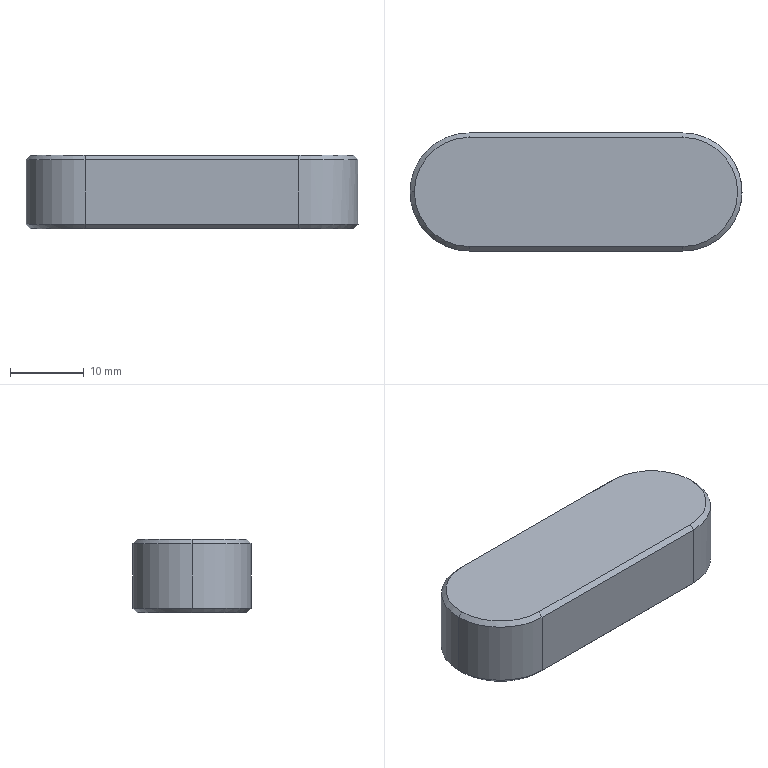Part | SolidWorks | features Boss 2, Chamfer 1, Extrusion 1 | 1 solid | 17 faces | box 45 x 16 x 10 mm | volume 6612 mm3 | plane 8 | cone 6 | cylinder 3 | commonest cylinder face diameters 16 x3
STEP:
#1=CARTESIAN_POINT('',(-36.4,0.,5.));
#2=VERTEX_POINT('',#1);
#3=CARTESIAN_POINT('',(-29.,-7.4,5.));
#4=VERTEX_POINT('',#3);
#5=CARTESIAN_POINT('',(-29.,0.,5.));
#6=DIRECTION('',(0.,0.,1.));
#7=DIRECTION('',(-1.,0.,0.));
#8=AXIS2_PLACEMENT_3D('',#5,#6,#7);
#9=CIRCLE('',#8,7.4);
#10=EDGE_CURVE('',#2,#4,#9,.T.);
#11=ORIENTED_EDGE('',*,*,#10,.F.);
#12=CARTESIAN_POINT('',(-37.,0.,4.4));
#13=VERTEX_POINT('',#12);
#14=CARTESIAN_POINT('',(-36.4,0.,5.));
#15=DIRECTION('',(-0.7071,0.,-0.7071));
#16=VECTOR('',#15,1000.);
#17=LINE('',#14,#16);
#18=EDGE_CURVE('',#2,#13,#17,.T.);
#19=ORIENTED_EDGE('',*,*,#18,.T.);
#20=CARTESIAN_POINT('',(-29.,-8.,4.4));
#21=VERTEX_POINT('',#20);
#22=CARTESIAN_POINT('',(-29.,0.,4.4));
#23=DIRECTION('',(0.,0.,-1.));
#24=DIRECTION('',(-1.,0.,0.));
#25=AXIS2_PLACEMENT_3D('',#22,#23,#24);
#26=CIRCLE('',#25,8.);
#27=EDGE_CURVE('',#21,#13,#26,.T.);
#28=ORIENTED_EDGE('',*,*,#27,.F.);
#29=CARTESIAN_POINT('',(-29.,-7.4,5.));
#30=DIRECTION('',(0.,-0.7071,-0.7071));
#31=VECTOR('',#30,1000.);
#32=LINE('',#29,#31);
#33=EDGE_CURVE('',#4,#21,#32,.T.);
#34=ORIENTED_EDGE('',*,*,#33,.F.);
#35=EDGE_LOOP('',(#11,#19,#28,#34));
#36=FACE_OUTER_BOUND('',#35,.T.);
#37=CARTESIAN_POINT('',(-29.,0.,5.));
#38=DIRECTION('',(0.,0.,-1.));
#39=DIRECTION('',(-1.,0.,0.));
#40=AXIS2_PLACEMENT_3D('',#37,#38,#39);
#41=CONICAL_SURFACE('',#40,7.4,0.7854);
#42=ADVANCED_FACE('',(#36),#41,.T.);
#43=CARTESIAN_POINT('',(7.4,0.,-5.));
#44=VERTEX_POINT('',#43);
#45=CARTESIAN_POINT('',(0.,-7.4,-5.));
#46=VERTEX_POINT('',#45);
#47=CARTESIAN_POINT('',(0.,0.,-5.));
#48=DIRECTION('',(0.,0.,-1.));
#49=DIRECTION('',(-1.,0.,0.));
#50=AXIS2_PLACEMENT_3D('',#47,#48,#49);
#51=CIRCLE('',#50,7.4);
#52=EDGE_CURVE('',#44,#46,#51,.T.);
#53=ORIENTED_EDGE('',*,*,#52,.F.);
#54=CARTESIAN_POINT('',(8.,0.,-4.4));
#55=VERTEX_POINT('',#54);
#56=CARTESIAN_POINT('',(8.,0.,-4.4));
#57=DIRECTION('',(0.7071,0.,0.7071));
#58=VECTOR('',#57,1000.);
#59=LINE('',#56,#58);
#60=EDGE_CURVE('',#44,#55,#59,.T.);
#61=ORIENTED_EDGE('',*,*,#60,.T.);
#62=CARTESIAN_POINT('',(0.,-8.,-4.4));
#63=VERTEX_POINT('',#62);
#64=CARTESIAN_POINT('',(0.,0.,-4.4));
#65=DIRECTION('',(0.,0.,1.));
#66=DIRECTION('',(-1.,0.,0.));
#67=AXIS2_PLACEMENT_3D('',#64,#65,#66);
#68=CIRCLE('',#67,8.);
#69=EDGE_CURVE('',#63,#55,#68,.T.);
#70=ORIENTED_EDGE('',*,*,#69,.F.);
#71=CARTESIAN_POINT('',(0.,-7.4,-5.));
#72=DIRECTION('',(0.,-0.7071,0.7071));
#73=VECTOR('',#72,1000.);
#74=LINE('',#71,#73);
#75=EDGE_CURVE('',#46,#63,#74,.T.);
#76=ORIENTED_EDGE('',*,*,#75,.F.);
#77=EDGE_LOOP('',(#53,#61,#70,#76));
#78=FACE_OUTER_BOUND('',#77,.T.);
#79=CARTESIAN_POINT('',(0.,0.,-4.4));
#80=DIRECTION('',(0.,0.,1.));
#81=DIRECTION('',(1.,0.,0.));
#82=AXIS2_PLACEMENT_3D('',#79,#80,#81);
#83=CONICAL_SURFACE('',#82,8.,0.7854);
#84=ADVANCED_FACE('',(#78),#83,.T.);
#85=ORIENTED_EDGE('',*,*,#27,.T.);
#86=CARTESIAN_POINT('',(-37.,0.,-4.4));
#87=VERTEX_POINT('',#86);
#88=CARTESIAN_POINT('',(-37.,0.,5.));
#89=DIRECTION('',(0.,0.,-1.));
#90=VECTOR('',#89,1000.);
#91=LINE('',#88,#90);
#92=EDGE_CURVE('',#13,#87,#91,.T.);
#93=ORIENTED_EDGE('',*,*,#92,.T.);
#94=CARTESIAN_POINT('',(-29.,-8.,-4.4));
#95=VERTEX_POINT('',#94);
#96=CARTESIAN_POINT('',(-29.,0.,-4.4));
#97=DIRECTION('',(0.,0.,1.));
#98=DIRECTION('',(-1.,0.,0.));
#99=AXIS2_PLACEMENT_3D('',#96,#97,#98);
#100=CIRCLE('',#99,8.);
#101=EDGE_CURVE('',#87,#95,#100,.T.);
#102=ORIENTED_EDGE('',*,*,#101,.T.);
#103=CARTESIAN_POINT('',(-29.,-8.,5.));
#104=DIRECTION('',(0.,0.,-1.));
#105=VECTOR('',#104,1000.);
#106=LINE('',#103,#105);
#107=EDGE_CURVE('',#21,#95,#106,.T.);
#108=ORIENTED_EDGE('',*,*,#107,.F.);
#109=EDGE_LOOP('',(#85,#93,#102,#108));
#110=FACE_OUTER_BOUND('',#109,.T.);
#111=CARTESIAN_POINT('',(-29.,0.,5.));
#112=DIRECTION('',(0.,0.,-1.));
#113=DIRECTION('',(-1.,0.,0.));
#114=AXIS2_PLACEMENT_3D('',#111,#112,#113);
#115=CYLINDRICAL_SURFACE('',#114,8.);
#116=ADVANCED_FACE('',(#110),#115,.T.);
#117=ORIENTED_EDGE('',*,*,#92,.F.);
#118=CARTESIAN_POINT('',(-29.,8.,4.4));
#119=VERTEX_POINT('',#118);
#120=CARTESIAN_POINT('',(-29.,0.,4.4));
#121=DIRECTION('',(0.,0.,-1.));
#122=DIRECTION('',(-1.,0.,0.));
#123=AXIS2_PLACEMENT_3D('',#120,#121,#122);
#124=CIRCLE('',#123,8.);
#125=EDGE_CURVE('',#13,#119,#124,.T.);
#126=ORIENTED_EDGE('',*,*,#125,.T.);
#127=CARTESIAN_POINT('',(-29.,8.,-4.4));
#128=VERTEX_POINT('',#127);
#129=CARTESIAN_POINT('',(-29.,8.,5.));
#130=DIRECTION('',(0.,0.,-1.));
#131=VECTOR('',#130,1000.);
#132=LINE('',#129,#131);
#133=EDGE_CURVE('',#119,#128,#132,.T.);
#134=ORIENTED_EDGE('',*,*,#133,.T.);
#135=CARTESIAN_POINT('',(-29.,0.,-4.4));
#136=DIRECTION('',(0.,0.,1.));
#137=DIRECTION('',(-1.,0.,0.));
#138=AXIS2_PLACEMENT_3D('',#135,#136,#137);
#139=CIRCLE('',#138,8.);
#140=EDGE_CURVE('',#128,#87,#139,.T.);
#141=ORIENTED_EDGE('',*,*,#140,.T.);
#142=EDGE_LOOP('',(#117,#126,#134,#141));
#143=FACE_OUTER_BOUND('',#142,.T.);
#144=CARTESIAN_POINT('',(-29.,0.,5.));
#145=DIRECTION('',(0.,0.,-1.));
#146=DIRECTION('',(-1.,0.,0.));
#147=AXIS2_PLACEMENT_3D('',#144,#145,#146);
#148=CYLINDRICAL_SURFACE('',#147,8.);
#149=ADVANCED_FACE('',(#143),#148,.T.);
#150=ORIENTED_EDGE('',*,*,#107,.T.);
#151=CARTESIAN_POINT('',(0.,-8.,-4.4));
#152=DIRECTION('',(1.,0.,0.));
#153=VECTOR('',#152,1000.);
#154=LINE('',#151,#153);
#155=EDGE_CURVE('',#95,#63,#154,.T.);
#156=ORIENTED_EDGE('',*,*,#155,.T.);
#157=CARTESIAN_POINT('',(0.,-8.,4.4));
#158=VERTEX_POINT('',#157);
#159=CARTESIAN_POINT('',(0.,-8.,5.));
#160=DIRECTION('',(0.,0.,-1.));
#161=VECTOR('',#160,1000.);
#162=LINE('',#159,#161);
#163=EDGE_CURVE('',#158,#63,#162,.T.);
#164=ORIENTED_EDGE('',*,*,#163,.F.);
#165=CARTESIAN_POINT('',(0.,-8.,4.4));
#166=DIRECTION('',(-1.,0.,0.));
#167=VECTOR('',#166,1000.);
#168=LINE('',#165,#167);
#169=EDGE_CURVE('',#158,#21,#168,.T.);
#170=ORIENTED_EDGE('',*,*,#169,.T.);
#171=EDGE_LOOP('',(#150,#156,#164,#170));
#172=FACE_OUTER_BOUND('',#171,.T.);
#173=CARTESIAN_POINT('',(0.,-8.,5.));
#174=DIRECTION('',(0.,1.,0.));
#175=DIRECTION('',(-1.,0.,0.));
#176=AXIS2_PLACEMENT_3D('',#173,#174,#175);
#177=PLANE('',#176);
#178=ADVANCED_FACE('',(#172),#177,.F.);
#179=CARTESIAN_POINT('',(0.,8.,4.4));
#180=VERTEX_POINT('',#179);
#181=CARTESIAN_POINT('',(0.,8.,-4.4));
#182=VERTEX_POINT('',#181);
#183=CARTESIAN_POINT('',(0.,8.,5.));
#184=DIRECTION('',(0.,0.,-1.));
#185=VECTOR('',#184,1000.);
#186=LINE('',#183,#185);
#187=EDGE_CURVE('',#180,#182,#186,.T.);
#188=ORIENTED_EDGE('',*,*,#187,.F.);
#189=CARTESIAN_POINT('',(0.,0.,4.4));
#190=DIRECTION('',(0.,0.,-1.));
#191=DIRECTION('',(-1.,0.,0.));
#192=AXIS2_PLACEMENT_3D('',#189,#190,#191);
#193=CIRCLE('',#192,8.);
#194=EDGE_CURVE('',#180,#158,#193,.T.);
#195=ORIENTED_EDGE('',*,*,#194,.T.);
#196=ORIENTED_EDGE('',*,*,#163,.T.);
#197=ORIENTED_EDGE('',*,*,#69,.T.);
#198=CARTESIAN_POINT('',(0.,0.,-4.4));
#199=DIRECTION('',(0.,0.,1.));
#200=DIRECTION('',(-1.,0.,0.));
#201=AXIS2_PLACEMENT_3D('',#198,#199,#200);
#202=CIRCLE('',#201,8.);
#203=EDGE_CURVE('',#55,#182,#202,.T.);
#204=ORIENTED_EDGE('',*,*,#203,.T.);
#205=EDGE_LOOP('',(#188,#195,#196,#197,#204));
#206=FACE_OUTER_BOUND('',#205,.T.);
#207=CARTESIAN_POINT('',(0.,0.,5.));
#208=DIRECTION('',(0.,0.,-1.));
#209=DIRECTION('',(-1.,0.,0.));
#210=AXIS2_PLACEMENT_3D('',#207,#208,#209);
#211=CYLINDRICAL_SURFACE('',#210,8.);
#212=ADVANCED_FACE('',(#206),#211,.T.);
#213=ORIENTED_EDGE('',*,*,#133,.F.);
#214=CARTESIAN_POINT('',(-29.,8.,4.4));
#215=DIRECTION('',(1.,0.,0.));
#216=VECTOR('',#215,1000.);
#217=LINE('',#214,#216);
#218=EDGE_CURVE('',#119,#180,#217,.T.);
#219=ORIENTED_EDGE('',*,*,#218,.T.);
#220=ORIENTED_EDGE('',*,*,#187,.T.);
#221=CARTESIAN_POINT('',(-29.,8.,-4.4));
#222=DIRECTION('',(-1.,0.,0.));
#223=VECTOR('',#222,1000.);
#224=LINE('',#221,#223);
#225=EDGE_CURVE('',#182,#128,#224,.T.);
#226=ORIENTED_EDGE('',*,*,#225,.T.);
#227=EDGE_LOOP('',(#213,#219,#220,#226));
#228=FACE_OUTER_BOUND('',#227,.T.);
#229=CARTESIAN_POINT('',(-29.,8.,5.));
#230=DIRECTION('',(0.,-1.,0.));
#231=DIRECTION('',(0.,0.,-1.));
#232=AXIS2_PLACEMENT_3D('',#229,#230,#231);
#233=PLANE('',#232);
#234=ADVANCED_FACE('',(#228),#233,.F.);
#235=CARTESIAN_POINT('',(-29.,7.4,5.));
#236=VERTEX_POINT('',#235);
#237=CARTESIAN_POINT('',(-29.,0.,5.));
#238=DIRECTION('',(0.,0.,1.));
#239=DIRECTION('',(-1.,0.,0.));
#240=AXIS2_PLACEMENT_3D('',#237,#238,#239);
#241=CIRCLE('',#240,7.4);
#242=EDGE_CURVE('',#236,#2,#241,.T.);
#243=ORIENTED_EDGE('',*,*,#242,.T.);
#244=ORIENTED_EDGE('',*,*,#10,.T.);
#245=CARTESIAN_POINT('',(0.,-7.4,5.));
#246=VERTEX_POINT('',#245);
#247=CARTESIAN_POINT('',(-29.,-7.4,5.));
#248=DIRECTION('',(1.,0.,0.));
#249=VECTOR('',#248,1000.);
#250=LINE('',#247,#249);
#251=EDGE_CURVE('',#4,#246,#250,.T.);
#252=ORIENTED_EDGE('',*,*,#251,.T.);
#253=CARTESIAN_POINT('',(0.,7.4,5.));
#254=VERTEX_POINT('',#253);
#255=CARTESIAN_POINT('',(0.,0.,5.));
#256=DIRECTION('',(0.,0.,1.));
#257=DIRECTION('',(-1.,0.,0.));
#258=AXIS2_PLACEMENT_3D('',#255,#256,#257);
#259=CIRCLE('',#258,7.4);
#260=EDGE_CURVE('',#246,#254,#259,.T.);
#261=ORIENTED_EDGE('',*,*,#260,.T.);
#262=CARTESIAN_POINT('',(-29.,7.4,5.));
#263=DIRECTION('',(-1.,0.,0.));
#264=VECTOR('',#263,1000.);
#265=LINE('',#262,#264);
#266=EDGE_CURVE('',#254,#236,#265,.T.);
#267=ORIENTED_EDGE('',*,*,#266,.T.);
#268=EDGE_LOOP('',(#243,#244,#252,#261,#267));
#269=FACE_OUTER_BOUND('',#268,.T.);
#270=CARTESIAN_POINT('',(-29.,0.,5.));
#271=DIRECTION('',(0.,0.,-1.));
#272=DIRECTION('',(-1.,0.,0.));
#273=AXIS2_PLACEMENT_3D('',#270,#271,#272);
#274=PLANE('',#273);
#275=ADVANCED_FACE('',(#269),#274,.F.);
#276=CARTESIAN_POINT('',(0.,7.4,-5.));
#277=VERTEX_POINT('',#276);
#278=CARTESIAN_POINT('',(0.,0.,-5.));
#279=DIRECTION('',(0.,0.,-1.));
#280=DIRECTION('',(-1.,0.,0.));
#281=AXIS2_PLACEMENT_3D('',#278,#279,#280);
#282=CIRCLE('',#281,7.4);
#283=EDGE_CURVE('',#277,#44,#282,.T.);
#284=ORIENTED_EDGE('',*,*,#283,.T.);
#285=ORIENTED_EDGE('',*,*,#52,.T.);
#286=CARTESIAN_POINT('',(-29.,-7.4,-5.));
#287=VERTEX_POINT('',#286);
#288=CARTESIAN_POINT('',(-29.,-7.4,-5.));
#289=DIRECTION('',(-1.,0.,0.));
#290=VECTOR('',#289,1000.);
#291=LINE('',#288,#290);
#292=EDGE_CURVE('',#46,#287,#291,.T.);
#293=ORIENTED_EDGE('',*,*,#292,.T.);
#294=CARTESIAN_POINT('',(-29.,7.4,-5.));
#295=VERTEX_POINT('',#294);
#296=CARTESIAN_POINT('',(-29.,0.,-5.));
#297=DIRECTION('',(0.,0.,-1.));
#298=DIRECTION('',(-1.,0.,0.));
#299=AXIS2_PLACEMENT_3D('',#296,#297,#298);
#300=CIRCLE('',#299,7.4);
#301=EDGE_CURVE('',#287,#295,#300,.T.);
#302=ORIENTED_EDGE('',*,*,#301,.T.);
#303=CARTESIAN_POINT('',(0.,7.4,-5.));
#304=DIRECTION('',(1.,0.,0.));
#305=VECTOR('',#304,1000.);
#306=LINE('',#303,#305);
#307=EDGE_CURVE('',#295,#277,#306,.T.);
#308=ORIENTED_EDGE('',*,*,#307,.T.);
#309=EDGE_LOOP('',(#284,#285,#293,#302,#308));
#310=FACE_OUTER_BOUND('',#309,.T.);
#311=CARTESIAN_POINT('',(-29.,0.,-5.));
#312=DIRECTION('',(0.,0.,-1.));
#313=DIRECTION('',(-1.,0.,0.));
#314=AXIS2_PLACEMENT_3D('',#311,#312,#313);
#315=PLANE('',#314);
#316=ADVANCED_FACE('',(#310),#315,.T.);
#317=CARTESIAN_POINT('',(0.,7.4,-5.));
#318=DIRECTION('',(0.,0.7071,0.7071));
#319=VECTOR('',#318,1000.);
#320=LINE('',#317,#319);
#321=EDGE_CURVE('',#277,#182,#320,.T.);
#322=ORIENTED_EDGE('',*,*,#321,.F.);
#323=ORIENTED_EDGE('',*,*,#307,.F.);
#324=CARTESIAN_POINT('',(-29.,8.,-4.4));
#325=DIRECTION('',(0.,-0.7071,-0.7071));
#326=VECTOR('',#325,1000.);
#327=LINE('',#324,#326);
#328=EDGE_CURVE('',#128,#295,#327,.T.);
#329=ORIENTED_EDGE('',*,*,#328,.F.);
#330=ORIENTED_EDGE('',*,*,#225,.F.);
#331=EDGE_LOOP('',(#322,#323,#329,#330));
#332=FACE_OUTER_BOUND('',#331,.T.);
#333=CARTESIAN_POINT('',(-29.,8.,-4.4));
#334=DIRECTION('',(0.,0.7071,-0.7071));
#335=DIRECTION('',(0.,0.7071,0.7071));
#336=AXIS2_PLACEMENT_3D('',#333,#334,#335);
#337=PLANE('',#336);
#338=ADVANCED_FACE('',(#332),#337,.T.);
#339=ORIENTED_EDGE('',*,*,#328,.T.);
#340=ORIENTED_EDGE('',*,*,#301,.F.);
#341=CARTESIAN_POINT('',(-29.,-8.,-4.4));
#342=DIRECTION('',(0.,0.7071,-0.7071));
#343=VECTOR('',#342,1000.);
#344=LINE('',#341,#343);
#345=EDGE_CURVE('',#95,#287,#344,.T.);
#346=ORIENTED_EDGE('',*,*,#345,.F.);
#347=ORIENTED_EDGE('',*,*,#101,.F.);
#348=ORIENTED_EDGE('',*,*,#140,.F.);
#349=EDGE_LOOP('',(#339,#340,#346,#347,#348));
#350=FACE_OUTER_BOUND('',#349,.T.);
#351=CARTESIAN_POINT('',(-29.,0.,-4.4));
#352=DIRECTION('',(0.,0.,1.));
#353=DIRECTION('',(1.,0.,0.));
#354=AXIS2_PLACEMENT_3D('',#351,#352,#353);
#355=CONICAL_SURFACE('',#354,8.,0.7854);
#356=ADVANCED_FACE('',(#350),#355,.T.);
#357=ORIENTED_EDGE('',*,*,#60,.F.);
#358=ORIENTED_EDGE('',*,*,#283,.F.);
#359=ORIENTED_EDGE('',*,*,#321,.T.);
#360=ORIENTED_EDGE('',*,*,#203,.F.);
#361=EDGE_LOOP('',(#357,#358,#359,#360));
#362=FACE_OUTER_BOUND('',#361,.T.);
#363=CARTESIAN_POINT('',(0.,0.,-4.4));
#364=DIRECTION('',(0.,0.,1.));
#365=DIRECTION('',(1.,0.,0.));
#366=AXIS2_PLACEMENT_3D('',#363,#364,#365);
#367=CONICAL_SURFACE('',#366,8.,0.7854);
#368=ADVANCED_FACE('',(#362),#367,.T.);
#369=ORIENTED_EDGE('',*,*,#345,.T.);
#370=ORIENTED_EDGE('',*,*,#292,.F.);
#371=ORIENTED_EDGE('',*,*,#75,.T.);
#372=ORIENTED_EDGE('',*,*,#155,.F.);
#373=EDGE_LOOP('',(#369,#370,#371,#372));
#374=FACE_OUTER_BOUND('',#373,.T.);
#375=CARTESIAN_POINT('',(0.,-8.,-4.4));
#376=DIRECTION('',(0.,-0.7071,-0.7071));
#377=DIRECTION('',(0.,0.7071,-0.7071));
#378=AXIS2_PLACEMENT_3D('',#375,#376,#377);
#379=PLANE('',#378);
#380=ADVANCED_FACE('',(#374),#379,.T.);
#381=CARTESIAN_POINT('',(0.,8.,4.4));
#382=DIRECTION('',(0.,-0.7071,0.7071));
#383=VECTOR('',#382,1000.);
#384=LINE('',#381,#383);
#385=EDGE_CURVE('',#180,#254,#384,.T.);
#386=ORIENTED_EDGE('',*,*,#385,.F.);
#387=ORIENTED_EDGE('',*,*,#218,.F.);
#388=CARTESIAN_POINT('',(-29.,7.4,5.));
#389=DIRECTION('',(0.,0.7071,-0.7071));
#390=VECTOR('',#389,1000.);
#391=LINE('',#388,#390);
#392=EDGE_CURVE('',#236,#119,#391,.T.);
#393=ORIENTED_EDGE('',*,*,#392,.F.);
#394=ORIENTED_EDGE('',*,*,#266,.F.);
#395=EDGE_LOOP('',(#386,#387,#393,#394));
#396=FACE_OUTER_BOUND('',#395,.T.);
#397=CARTESIAN_POINT('',(-29.,7.4,5.));
#398=DIRECTION('',(0.,-0.7071,-0.7071));
#399=DIRECTION('',(0.,0.7071,-0.7071));
#400=AXIS2_PLACEMENT_3D('',#397,#398,#399);
#401=PLANE('',#400);
#402=ADVANCED_FACE('',(#396),#401,.F.);
#403=ORIENTED_EDGE('',*,*,#18,.F.);
#404=ORIENTED_EDGE('',*,*,#242,.F.);
#405=ORIENTED_EDGE('',*,*,#392,.T.);
#406=ORIENTED_EDGE('',*,*,#125,.F.);
#407=EDGE_LOOP('',(#403,#404,#405,#406));
#408=FACE_OUTER_BOUND('',#407,.T.);
#409=CARTESIAN_POINT('',(-29.,0.,5.));
#410=DIRECTION('',(0.,0.,-1.));
#411=DIRECTION('',(-1.,0.,0.));
#412=AXIS2_PLACEMENT_3D('',#409,#410,#411);
#413=CONICAL_SURFACE('',#412,7.4,0.7854);
#414=ADVANCED_FACE('',(#408),#413,.T.);
#415=ORIENTED_EDGE('',*,*,#385,.T.);
#416=ORIENTED_EDGE('',*,*,#260,.F.);
#417=CARTESIAN_POINT('',(0.,-8.,4.4));
#418=DIRECTION('',(0.,0.7071,0.7071));
#419=VECTOR('',#418,1000.);
#420=LINE('',#417,#419);
#421=EDGE_CURVE('',#158,#246,#420,.T.);
#422=ORIENTED_EDGE('',*,*,#421,.F.);
#423=ORIENTED_EDGE('',*,*,#194,.F.);
#424=EDGE_LOOP('',(#415,#416,#422,#423));
#425=FACE_OUTER_BOUND('',#424,.T.);
#426=CARTESIAN_POINT('',(0.,0.,5.));
#427=DIRECTION('',(0.,0.,-1.));
#428=DIRECTION('',(-1.,0.,0.));
#429=AXIS2_PLACEMENT_3D('',#426,#427,#428);
#430=CONICAL_SURFACE('',#429,7.4,0.7854);
#431=ADVANCED_FACE('',(#425),#430,.T.);
#432=ORIENTED_EDGE('',*,*,#33,.T.);
#433=ORIENTED_EDGE('',*,*,#169,.F.);
#434=ORIENTED_EDGE('',*,*,#421,.T.);
#435=ORIENTED_EDGE('',*,*,#251,.F.);
#436=EDGE_LOOP('',(#432,#433,#434,#435));
#437=FACE_OUTER_BOUND('',#436,.T.);
#438=CARTESIAN_POINT('',(-29.,-7.4,5.));
#439=DIRECTION('',(0.,0.7071,-0.7071));
#440=DIRECTION('',(0.,0.7071,0.7071));
#441=AXIS2_PLACEMENT_3D('',#438,#439,#440);
#442=PLANE('',#441);
#443=ADVANCED_FACE('',(#437),#442,.F.);
#444=CLOSED_SHELL('',(#42,#84,#116,#149,#178,#212,#234,#275,#316,#338,#356,#368,#380,#402,#414,#431,#443));
#445=MANIFOLD_SOLID_BREP('',#444);
#446=CARTESIAN_POINT('',(0.,0.,0.));
#447=DIRECTION('',(0.,0.,1.));
#448=DIRECTION('',(1.,0.,0.));
#449=AXIS2_PLACEMENT_3D('',#446,#447,#448);
#450=(LENGTH_UNIT()NAMED_UNIT(*)SI_UNIT(.MILLI.,.METRE.));
#451=UNCERTAINTY_MEASURE_WITH_UNIT(LENGTH_MEASURE(0.00001),#450,'','');
#452=(NAMED_UNIT(*)PLANE_ANGLE_UNIT()SI_UNIT($,.RADIAN.));
#453=(NAMED_UNIT(*)SI_UNIT($,.STERADIAN.)SOLID_ANGLE_UNIT());
#454=(GEOMETRIC_REPRESENTATION_CONTEXT(3)GLOBAL_UNCERTAINTY_ASSIGNED_CONTEXT((#451))GLOBAL_UNIT_ASSIGNED_CONTEXT((#450,#452,#453))REPRESENTATION_CONTEXT('',''));
#455=ADVANCED_BREP_SHAPE_REPRESENTATION('',(#445,#449),#454);